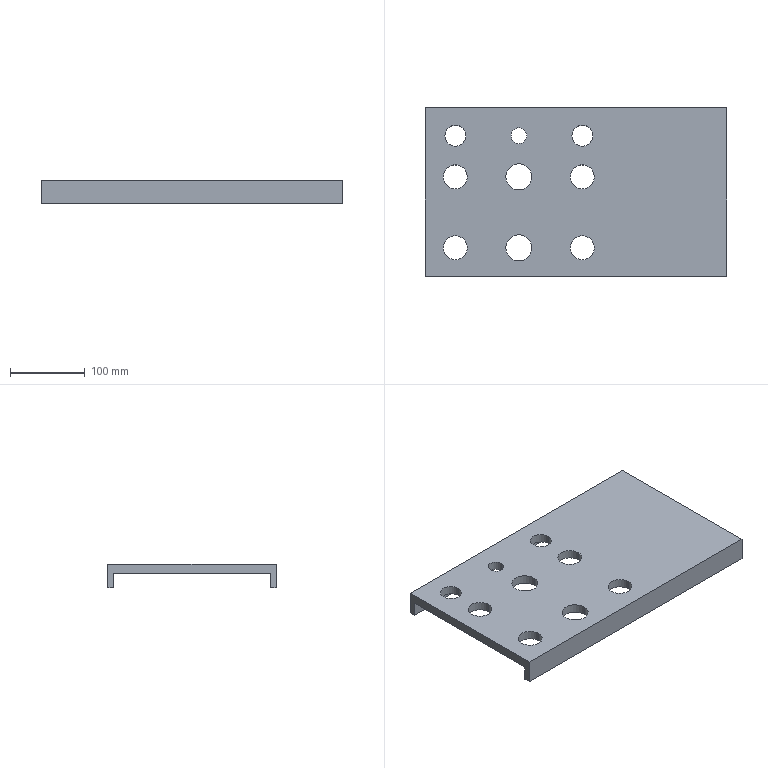Part | SolidWorks | features ICE 3, MoveFace 2, Extrusion 1 | 1 solid | 28 faces | box 403 x 225.5 x 32 mm | volume 1138849 mm3 | cylinder 18 | plane 10 | commonest cylinder face diameters 32 x8 28 x4 35 x4 21 x2
STEP:
#1=CARTESIAN_POINT('',(71.,80.,0.));
#2=VERTEX_POINT('',#1);
#3=CARTESIAN_POINT('',(99.,80.,0.));
#4=VERTEX_POINT('',#3);
#5=CARTESIAN_POINT('',(85.,80.,0.));
#6=DIRECTION('',(0.,0.,1.));
#7=DIRECTION('',(-1.,0.,0.));
#8=AXIS2_PLACEMENT_3D('',#5,#6,#7);
#9=CIRCLE('',#8,14.);
#10=EDGE_CURVE('',#2,#4,#9,.T.);
#11=ORIENTED_EDGE('',*,*,#10,.F.);
#12=CARTESIAN_POINT('',(71.,80.,12.));
#13=VERTEX_POINT('',#12);
#14=CARTESIAN_POINT('',(71.,80.,-0.001));
#15=DIRECTION('',(0.,0.,1.));
#16=VECTOR('',#15,1000.);
#17=LINE('',#14,#16);
#18=EDGE_CURVE('',#2,#13,#17,.T.);
#19=ORIENTED_EDGE('',*,*,#18,.T.);
#20=CARTESIAN_POINT('',(99.,80.,12.));
#21=VERTEX_POINT('',#20);
#22=CARTESIAN_POINT('',(85.,80.,12.));
#23=DIRECTION('',(0.,0.,1.));
#24=DIRECTION('',(1.,0.,0.));
#25=AXIS2_PLACEMENT_3D('',#22,#23,#24);
#26=CIRCLE('',#25,14.);
#27=EDGE_CURVE('',#13,#21,#26,.T.);
#28=ORIENTED_EDGE('',*,*,#27,.T.);
#29=CARTESIAN_POINT('',(99.,80.,-0.001));
#30=DIRECTION('',(0.,0.,1.));
#31=VECTOR('',#30,1000.);
#32=LINE('',#29,#31);
#33=EDGE_CURVE('',#4,#21,#32,.T.);
#34=ORIENTED_EDGE('',*,*,#33,.F.);
#35=EDGE_LOOP('',(#11,#19,#28,#34));
#36=FACE_OUTER_BOUND('',#35,.T.);
#37=CARTESIAN_POINT('',(85.,80.,-0.001));
#38=DIRECTION('',(0.,0.,1.));
#39=DIRECTION('',(1.,0.,0.));
#40=AXIS2_PLACEMENT_3D('',#37,#38,#39);
#41=CYLINDRICAL_SURFACE('',#40,14.);
#42=ADVANCED_FACE('',(#36),#41,.F.);
#43=CARTESIAN_POINT('',(-99.,80.,0.));
#44=VERTEX_POINT('',#43);
#45=CARTESIAN_POINT('',(-71.,80.,0.));
#46=VERTEX_POINT('',#45);
#47=CARTESIAN_POINT('',(-85.,80.,0.));
#48=DIRECTION('',(0.,0.,1.));
#49=DIRECTION('',(-1.,0.,0.));
#50=AXIS2_PLACEMENT_3D('',#47,#48,#49);
#51=CIRCLE('',#50,14.);
#52=EDGE_CURVE('',#44,#46,#51,.T.);
#53=ORIENTED_EDGE('',*,*,#52,.F.);
#54=CARTESIAN_POINT('',(-99.,80.,12.));
#55=VERTEX_POINT('',#54);
#56=CARTESIAN_POINT('',(-99.,80.,-0.001));
#57=DIRECTION('',(0.,0.,1.));
#58=VECTOR('',#57,1000.);
#59=LINE('',#56,#58);
#60=EDGE_CURVE('',#44,#55,#59,.T.);
#61=ORIENTED_EDGE('',*,*,#60,.T.);
#62=CARTESIAN_POINT('',(-71.,80.,12.));
#63=VERTEX_POINT('',#62);
#64=CARTESIAN_POINT('',(-85.,80.,12.));
#65=DIRECTION('',(0.,0.,1.));
#66=DIRECTION('',(1.,0.,0.));
#67=AXIS2_PLACEMENT_3D('',#64,#65,#66);
#68=CIRCLE('',#67,14.);
#69=EDGE_CURVE('',#55,#63,#68,.T.);
#70=ORIENTED_EDGE('',*,*,#69,.T.);
#71=CARTESIAN_POINT('',(-71.,80.,-0.001));
#72=DIRECTION('',(0.,0.,1.));
#73=VECTOR('',#72,1000.);
#74=LINE('',#71,#73);
#75=EDGE_CURVE('',#46,#63,#74,.T.);
#76=ORIENTED_EDGE('',*,*,#75,.F.);
#77=EDGE_LOOP('',(#53,#61,#70,#76));
#78=FACE_OUTER_BOUND('',#77,.T.);
#79=CARTESIAN_POINT('',(-85.,80.,-0.001));
#80=DIRECTION('',(0.,0.,1.));
#81=DIRECTION('',(1.,0.,0.));
#82=AXIS2_PLACEMENT_3D('',#79,#80,#81);
#83=CYLINDRICAL_SURFACE('',#82,14.);
#84=ADVANCED_FACE('',(#78),#83,.F.);
#85=CARTESIAN_POINT('',(-17.5,25.,0.));
#86=VERTEX_POINT('',#85);
#87=CARTESIAN_POINT('',(17.5,25.,0.));
#88=VERTEX_POINT('',#87);
#89=CARTESIAN_POINT('',(0.,25.,0.));
#90=DIRECTION('',(0.,0.,1.));
#91=DIRECTION('',(-1.,0.,0.));
#92=AXIS2_PLACEMENT_3D('',#89,#90,#91);
#93=CIRCLE('',#92,17.5);
#94=EDGE_CURVE('',#86,#88,#93,.T.);
#95=ORIENTED_EDGE('',*,*,#94,.F.);
#96=CARTESIAN_POINT('',(-17.5,25.,12.));
#97=VERTEX_POINT('',#96);
#98=CARTESIAN_POINT('',(-17.5,25.,-0.001));
#99=DIRECTION('',(0.,0.,1.));
#100=VECTOR('',#99,1000.);
#101=LINE('',#98,#100);
#102=EDGE_CURVE('',#86,#97,#101,.T.);
#103=ORIENTED_EDGE('',*,*,#102,.T.);
#104=CARTESIAN_POINT('',(17.5,25.,12.));
#105=VERTEX_POINT('',#104);
#106=CARTESIAN_POINT('',(0.,25.,12.));
#107=DIRECTION('',(0.,0.,1.));
#108=DIRECTION('',(1.,0.,0.));
#109=AXIS2_PLACEMENT_3D('',#106,#107,#108);
#110=CIRCLE('',#109,17.5);
#111=EDGE_CURVE('',#97,#105,#110,.T.);
#112=ORIENTED_EDGE('',*,*,#111,.T.);
#113=CARTESIAN_POINT('',(17.5,25.,-0.001));
#114=DIRECTION('',(0.,0.,1.));
#115=VECTOR('',#114,1000.);
#116=LINE('',#113,#115);
#117=EDGE_CURVE('',#88,#105,#116,.T.);
#118=ORIENTED_EDGE('',*,*,#117,.F.);
#119=EDGE_LOOP('',(#95,#103,#112,#118));
#120=FACE_OUTER_BOUND('',#119,.T.);
#121=CARTESIAN_POINT('',(0.,25.,-0.001));
#122=DIRECTION('',(0.,0.,1.));
#123=DIRECTION('',(1.,0.,0.));
#124=AXIS2_PLACEMENT_3D('',#121,#122,#123);
#125=CYLINDRICAL_SURFACE('',#124,17.5);
#126=ADVANCED_FACE('',(#120),#125,.F.);
#127=CARTESIAN_POINT('',(-101.,25.,0.));
#128=VERTEX_POINT('',#127);
#129=CARTESIAN_POINT('',(-69.,25.,0.));
#130=VERTEX_POINT('',#129);
#131=CARTESIAN_POINT('',(-85.,25.,0.));
#132=DIRECTION('',(0.,0.,1.));
#133=DIRECTION('',(-1.,0.,0.));
#134=AXIS2_PLACEMENT_3D('',#131,#132,#133);
#135=CIRCLE('',#134,16.);
#136=EDGE_CURVE('',#128,#130,#135,.T.);
#137=ORIENTED_EDGE('',*,*,#136,.F.);
#138=CARTESIAN_POINT('',(-101.,25.,12.));
#139=VERTEX_POINT('',#138);
#140=CARTESIAN_POINT('',(-101.,25.,-0.001));
#141=DIRECTION('',(0.,0.,1.));
#142=VECTOR('',#141,1000.);
#143=LINE('',#140,#142);
#144=EDGE_CURVE('',#128,#139,#143,.T.);
#145=ORIENTED_EDGE('',*,*,#144,.T.);
#146=CARTESIAN_POINT('',(-69.,25.,12.));
#147=VERTEX_POINT('',#146);
#148=CARTESIAN_POINT('',(-85.,25.,12.));
#149=DIRECTION('',(0.,0.,1.));
#150=DIRECTION('',(1.,0.,0.));
#151=AXIS2_PLACEMENT_3D('',#148,#149,#150);
#152=CIRCLE('',#151,16.);
#153=EDGE_CURVE('',#139,#147,#152,.T.);
#154=ORIENTED_EDGE('',*,*,#153,.T.);
#155=CARTESIAN_POINT('',(-69.,25.,-0.001));
#156=DIRECTION('',(0.,0.,1.));
#157=VECTOR('',#156,1000.);
#158=LINE('',#155,#157);
#159=EDGE_CURVE('',#130,#147,#158,.T.);
#160=ORIENTED_EDGE('',*,*,#159,.F.);
#161=EDGE_LOOP('',(#137,#145,#154,#160));
#162=FACE_OUTER_BOUND('',#161,.T.);
#163=CARTESIAN_POINT('',(-85.,25.,-0.001));
#164=DIRECTION('',(0.,0.,1.));
#165=DIRECTION('',(1.,0.,0.));
#166=AXIS2_PLACEMENT_3D('',#163,#164,#165);
#167=CYLINDRICAL_SURFACE('',#166,16.);
#168=ADVANCED_FACE('',(#162),#167,.F.);
#169=CARTESIAN_POINT('',(-101.,-70.,0.));
#170=VERTEX_POINT('',#169);
#171=CARTESIAN_POINT('',(-69.,-70.,0.));
#172=VERTEX_POINT('',#171);
#173=CARTESIAN_POINT('',(-85.,-70.,0.));
#174=DIRECTION('',(0.,0.,1.));
#175=DIRECTION('',(-1.,0.,0.));
#176=AXIS2_PLACEMENT_3D('',#173,#174,#175);
#177=CIRCLE('',#176,16.);
#178=EDGE_CURVE('',#170,#172,#177,.T.);
#179=ORIENTED_EDGE('',*,*,#178,.F.);
#180=CARTESIAN_POINT('',(-101.,-70.,12.));
#181=VERTEX_POINT('',#180);
#182=CARTESIAN_POINT('',(-101.,-70.,-0.001));
#183=DIRECTION('',(0.,0.,1.));
#184=VECTOR('',#183,1000.);
#185=LINE('',#182,#184);
#186=EDGE_CURVE('',#170,#181,#185,.T.);
#187=ORIENTED_EDGE('',*,*,#186,.T.);
#188=CARTESIAN_POINT('',(-69.,-70.,12.));
#189=VERTEX_POINT('',#188);
#190=CARTESIAN_POINT('',(-85.,-70.,12.));
#191=DIRECTION('',(0.,0.,1.));
#192=DIRECTION('',(1.,0.,0.));
#193=AXIS2_PLACEMENT_3D('',#190,#191,#192);
#194=CIRCLE('',#193,16.);
#195=EDGE_CURVE('',#181,#189,#194,.T.);
#196=ORIENTED_EDGE('',*,*,#195,.T.);
#197=CARTESIAN_POINT('',(-69.,-70.,-0.001));
#198=DIRECTION('',(0.,0.,1.));
#199=VECTOR('',#198,1000.);
#200=LINE('',#197,#199);
#201=EDGE_CURVE('',#172,#189,#200,.T.);
#202=ORIENTED_EDGE('',*,*,#201,.F.);
#203=EDGE_LOOP('',(#179,#187,#196,#202));
#204=FACE_OUTER_BOUND('',#203,.T.);
#205=CARTESIAN_POINT('',(-85.,-70.,-0.001));
#206=DIRECTION('',(0.,0.,1.));
#207=DIRECTION('',(1.,0.,0.));
#208=AXIS2_PLACEMENT_3D('',#205,#206,#207);
#209=CYLINDRICAL_SURFACE('',#208,16.);
#210=ADVANCED_FACE('',(#204),#209,.F.);
#211=CARTESIAN_POINT('',(69.,-70.,0.));
#212=VERTEX_POINT('',#211);
#213=CARTESIAN_POINT('',(101.,-70.,0.));
#214=VERTEX_POINT('',#213);
#215=CARTESIAN_POINT('',(85.,-70.,0.));
#216=DIRECTION('',(0.,0.,1.));
#217=DIRECTION('',(-1.,0.,0.));
#218=AXIS2_PLACEMENT_3D('',#215,#216,#217);
#219=CIRCLE('',#218,16.);
#220=EDGE_CURVE('',#212,#214,#219,.T.);
#221=ORIENTED_EDGE('',*,*,#220,.F.);
#222=CARTESIAN_POINT('',(69.,-70.,12.));
#223=VERTEX_POINT('',#222);
#224=CARTESIAN_POINT('',(69.,-70.,-0.001));
#225=DIRECTION('',(0.,0.,1.));
#226=VECTOR('',#225,1000.);
#227=LINE('',#224,#226);
#228=EDGE_CURVE('',#212,#223,#227,.T.);
#229=ORIENTED_EDGE('',*,*,#228,.T.);
#230=CARTESIAN_POINT('',(101.,-70.,12.));
#231=VERTEX_POINT('',#230);
#232=CARTESIAN_POINT('',(85.,-70.,12.));
#233=DIRECTION('',(0.,0.,1.));
#234=DIRECTION('',(1.,0.,0.));
#235=AXIS2_PLACEMENT_3D('',#232,#233,#234);
#236=CIRCLE('',#235,16.);
#237=EDGE_CURVE('',#223,#231,#236,.T.);
#238=ORIENTED_EDGE('',*,*,#237,.T.);
#239=CARTESIAN_POINT('',(101.,-70.,-0.001));
#240=DIRECTION('',(0.,0.,1.));
#241=VECTOR('',#240,1000.);
#242=LINE('',#239,#241);
#243=EDGE_CURVE('',#214,#231,#242,.T.);
#244=ORIENTED_EDGE('',*,*,#243,.F.);
#245=EDGE_LOOP('',(#221,#229,#238,#244));
#246=FACE_OUTER_BOUND('',#245,.T.);
#247=CARTESIAN_POINT('',(85.,-70.,-0.001));
#248=DIRECTION('',(0.,0.,1.));
#249=DIRECTION('',(1.,0.,0.));
#250=AXIS2_PLACEMENT_3D('',#247,#248,#249);
#251=CYLINDRICAL_SURFACE('',#250,16.);
#252=ADVANCED_FACE('',(#246),#251,.F.);
#253=CARTESIAN_POINT('',(-17.5,-70.,0.));
#254=VERTEX_POINT('',#253);
#255=CARTESIAN_POINT('',(17.5,-70.,0.));
#256=VERTEX_POINT('',#255);
#257=CARTESIAN_POINT('',(0.,-70.,0.));
#258=DIRECTION('',(0.,0.,1.));
#259=DIRECTION('',(-1.,0.,0.));
#260=AXIS2_PLACEMENT_3D('',#257,#258,#259);
#261=CIRCLE('',#260,17.5);
#262=EDGE_CURVE('',#254,#256,#261,.T.);
#263=ORIENTED_EDGE('',*,*,#262,.F.);
#264=CARTESIAN_POINT('',(-17.5,-70.,12.));
#265=VERTEX_POINT('',#264);
#266=CARTESIAN_POINT('',(-17.5,-70.,-0.001));
#267=DIRECTION('',(0.,0.,1.));
#268=VECTOR('',#267,1000.);
#269=LINE('',#266,#268);
#270=EDGE_CURVE('',#254,#265,#269,.T.);
#271=ORIENTED_EDGE('',*,*,#270,.T.);
#272=CARTESIAN_POINT('',(17.5,-70.,12.));
#273=VERTEX_POINT('',#272);
#274=CARTESIAN_POINT('',(0.,-70.,12.));
#275=DIRECTION('',(0.,0.,1.));
#276=DIRECTION('',(1.,0.,0.));
#277=AXIS2_PLACEMENT_3D('',#274,#275,#276);
#278=CIRCLE('',#277,17.5);
#279=EDGE_CURVE('',#265,#273,#278,.T.);
#280=ORIENTED_EDGE('',*,*,#279,.T.);
#281=CARTESIAN_POINT('',(17.5,-70.,-0.001));
#282=DIRECTION('',(0.,0.,1.));
#283=VECTOR('',#282,1000.);
#284=LINE('',#281,#283);
#285=EDGE_CURVE('',#256,#273,#284,.T.);
#286=ORIENTED_EDGE('',*,*,#285,.F.);
#287=EDGE_LOOP('',(#263,#271,#280,#286));
#288=FACE_OUTER_BOUND('',#287,.T.);
#289=CARTESIAN_POINT('',(0.,-70.,-0.001));
#290=DIRECTION('',(0.,0.,1.));
#291=DIRECTION('',(1.,0.,0.));
#292=AXIS2_PLACEMENT_3D('',#289,#290,#291);
#293=CYLINDRICAL_SURFACE('',#292,17.5);
#294=ADVANCED_FACE('',(#288),#293,.F.);
#295=CARTESIAN_POINT('',(69.,25.,0.));
#296=VERTEX_POINT('',#295);
#297=CARTESIAN_POINT('',(101.,25.,0.));
#298=VERTEX_POINT('',#297);
#299=CARTESIAN_POINT('',(85.,25.,0.));
#300=DIRECTION('',(0.,0.,1.));
#301=DIRECTION('',(-1.,0.,0.));
#302=AXIS2_PLACEMENT_3D('',#299,#300,#301);
#303=CIRCLE('',#302,16.);
#304=EDGE_CURVE('',#296,#298,#303,.T.);
#305=ORIENTED_EDGE('',*,*,#304,.F.);
#306=CARTESIAN_POINT('',(69.,25.,12.));
#307=VERTEX_POINT('',#306);
#308=CARTESIAN_POINT('',(69.,25.,-0.001));
#309=DIRECTION('',(0.,0.,1.));
#310=VECTOR('',#309,1000.);
#311=LINE('',#308,#310);
#312=EDGE_CURVE('',#296,#307,#311,.T.);
#313=ORIENTED_EDGE('',*,*,#312,.T.);
#314=CARTESIAN_POINT('',(101.,25.,12.));
#315=VERTEX_POINT('',#314);
#316=CARTESIAN_POINT('',(85.,25.,12.));
#317=DIRECTION('',(0.,0.,1.));
#318=DIRECTION('',(1.,0.,0.));
#319=AXIS2_PLACEMENT_3D('',#316,#317,#318);
#320=CIRCLE('',#319,16.);
#321=EDGE_CURVE('',#307,#315,#320,.T.);
#322=ORIENTED_EDGE('',*,*,#321,.T.);
#323=CARTESIAN_POINT('',(101.,25.,-0.001));
#324=DIRECTION('',(0.,0.,1.));
#325=VECTOR('',#324,1000.);
#326=LINE('',#323,#325);
#327=EDGE_CURVE('',#298,#315,#326,.T.);
#328=ORIENTED_EDGE('',*,*,#327,.F.);
#329=EDGE_LOOP('',(#305,#313,#322,#328));
#330=FACE_OUTER_BOUND('',#329,.T.);
#331=CARTESIAN_POINT('',(85.,25.,-0.001));
#332=DIRECTION('',(0.,0.,1.));
#333=DIRECTION('',(1.,0.,0.));
#334=AXIS2_PLACEMENT_3D('',#331,#332,#333);
#335=CYLINDRICAL_SURFACE('',#334,16.);
#336=ADVANCED_FACE('',(#330),#335,.F.);
#337=CARTESIAN_POINT('',(-10.5,80.,0.));
#338=VERTEX_POINT('',#337);
#339=CARTESIAN_POINT('',(10.5,80.,0.));
#340=VERTEX_POINT('',#339);
#341=CARTESIAN_POINT('',(0.,80.,0.));
#342=DIRECTION('',(0.,0.,1.));
#343=DIRECTION('',(-1.,0.,0.));
#344=AXIS2_PLACEMENT_3D('',#341,#342,#343);
#345=CIRCLE('',#344,10.5);
#346=EDGE_CURVE('',#338,#340,#345,.T.);
#347=ORIENTED_EDGE('',*,*,#346,.F.);
#348=CARTESIAN_POINT('',(-10.5,80.,12.));
#349=VERTEX_POINT('',#348);
#350=CARTESIAN_POINT('',(-10.5,80.,-0.001));
#351=DIRECTION('',(0.,0.,1.));
#352=VECTOR('',#351,1000.);
#353=LINE('',#350,#352);
#354=EDGE_CURVE('',#338,#349,#353,.T.);
#355=ORIENTED_EDGE('',*,*,#354,.T.);
#356=CARTESIAN_POINT('',(10.5,80.,12.));
#357=VERTEX_POINT('',#356);
#358=CARTESIAN_POINT('',(0.,80.,12.));
#359=DIRECTION('',(0.,0.,1.));
#360=DIRECTION('',(1.,0.,0.));
#361=AXIS2_PLACEMENT_3D('',#358,#359,#360);
#362=CIRCLE('',#361,10.5);
#363=EDGE_CURVE('',#349,#357,#362,.T.);
#364=ORIENTED_EDGE('',*,*,#363,.T.);
#365=CARTESIAN_POINT('',(10.5,80.,-0.001));
#366=DIRECTION('',(0.,0.,1.));
#367=VECTOR('',#366,1000.);
#368=LINE('',#365,#367);
#369=EDGE_CURVE('',#340,#357,#368,.T.);
#370=ORIENTED_EDGE('',*,*,#369,.F.);
#371=EDGE_LOOP('',(#347,#355,#364,#370));
#372=FACE_OUTER_BOUND('',#371,.T.);
#373=CARTESIAN_POINT('',(0.,80.,-0.001));
#374=DIRECTION('',(0.,0.,1.));
#375=DIRECTION('',(1.,0.,0.));
#376=AXIS2_PLACEMENT_3D('',#373,#374,#375);
#377=CYLINDRICAL_SURFACE('',#376,10.5);
#378=ADVANCED_FACE('',(#372),#377,.F.);
#379=CARTESIAN_POINT('',(85.,80.,0.));
#380=DIRECTION('',(0.,0.,1.));
#381=DIRECTION('',(-1.,0.,0.));
#382=AXIS2_PLACEMENT_3D('',#379,#380,#381);
#383=CIRCLE('',#382,14.);
#384=EDGE_CURVE('',#4,#2,#383,.T.);
#385=ORIENTED_EDGE('',*,*,#384,.T.);
#386=ORIENTED_EDGE('',*,*,#10,.T.);
#387=EDGE_LOOP('',(#385,#386));
#388=FACE_BOUND('',#387,.T.);
#389=CARTESIAN_POINT('',(-85.,80.,0.));
#390=DIRECTION('',(0.,0.,1.));
#391=DIRECTION('',(-1.,0.,0.));
#392=AXIS2_PLACEMENT_3D('',#389,#390,#391);
#393=CIRCLE('',#392,14.);
#394=EDGE_CURVE('',#46,#44,#393,.T.);
#395=ORIENTED_EDGE('',*,*,#394,.T.);
#396=ORIENTED_EDGE('',*,*,#52,.T.);
#397=EDGE_LOOP('',(#395,#396));
#398=FACE_BOUND('',#397,.T.);
#399=CARTESIAN_POINT('',(0.,25.,0.));
#400=DIRECTION('',(0.,0.,1.));
#401=DIRECTION('',(-1.,0.,0.));
#402=AXIS2_PLACEMENT_3D('',#399,#400,#401);
#403=CIRCLE('',#402,17.5);
#404=EDGE_CURVE('',#88,#86,#403,.T.);
#405=ORIENTED_EDGE('',*,*,#404,.T.);
#406=ORIENTED_EDGE('',*,*,#94,.T.);
#407=EDGE_LOOP('',(#405,#406));
#408=FACE_BOUND('',#407,.T.);
#409=CARTESIAN_POINT('',(-85.,25.,0.));
#410=DIRECTION('',(0.,0.,1.));
#411=DIRECTION('',(-1.,0.,0.));
#412=AXIS2_PLACEMENT_3D('',#409,#410,#411);
#413=CIRCLE('',#412,16.);
#414=EDGE_CURVE('',#130,#128,#413,.T.);
#415=ORIENTED_EDGE('',*,*,#414,.T.);
#416=ORIENTED_EDGE('',*,*,#136,.T.);
#417=EDGE_LOOP('',(#415,#416));
#418=FACE_BOUND('',#417,.T.);
#419=CARTESIAN_POINT('',(-85.,-70.,0.));
#420=DIRECTION('',(0.,0.,1.));
#421=DIRECTION('',(-1.,0.,0.));
#422=AXIS2_PLACEMENT_3D('',#419,#420,#421);
#423=CIRCLE('',#422,16.);
#424=EDGE_CURVE('',#172,#170,#423,.T.);
#425=ORIENTED_EDGE('',*,*,#424,.T.);
#426=ORIENTED_EDGE('',*,*,#178,.T.);
#427=EDGE_LOOP('',(#425,#426));
#428=FACE_BOUND('',#427,.T.);
#429=CARTESIAN_POINT('',(85.,-70.,0.));
#430=DIRECTION('',(0.,0.,1.));
#431=DIRECTION('',(-1.,0.,0.));
#432=AXIS2_PLACEMENT_3D('',#429,#430,#431);
#433=CIRCLE('',#432,16.);
#434=EDGE_CURVE('',#214,#212,#433,.T.);
#435=ORIENTED_EDGE('',*,*,#434,.T.);
#436=ORIENTED_EDGE('',*,*,#220,.T.);
#437=EDGE_LOOP('',(#435,#436));
#438=FACE_BOUND('',#437,.T.);
#439=CARTESIAN_POINT('',(0.,-70.,0.));
#440=DIRECTION('',(0.,0.,1.));
#441=DIRECTION('',(-1.,0.,0.));
#442=AXIS2_PLACEMENT_3D('',#439,#440,#441);
#443=CIRCLE('',#442,17.5);
#444=EDGE_CURVE('',#256,#254,#443,.T.);
#445=ORIENTED_EDGE('',*,*,#444,.T.);
#446=ORIENTED_EDGE('',*,*,#262,.T.);
#447=EDGE_LOOP('',(#445,#446));
#448=FACE_BOUND('',#447,.T.);
#449=CARTESIAN_POINT('',(85.,25.,0.));
#450=DIRECTION('',(0.,0.,1.));
#451=DIRECTION('',(-1.,0.,0.));
#452=AXIS2_PLACEMENT_3D('',#449,#450,#451);
#453=CIRCLE('',#452,16.);
#454=EDGE_CURVE('',#298,#296,#453,.T.);
#455=ORIENTED_EDGE('',*,*,#454,.T.);
#456=ORIENTED_EDGE('',*,*,#304,.T.);
#457=EDGE_LOOP('',(#455,#456));
#458=FACE_BOUND('',#457,.T.);
#459=CARTESIAN_POINT('',(0.,80.,0.));
#460=DIRECTION('',(0.,0.,1.));
#461=DIRECTION('',(-1.,0.,0.));
#462=AXIS2_PLACEMENT_3D('',#459,#460,#461);
#463=CIRCLE('',#462,10.5);
#464=EDGE_CURVE('',#340,#338,#463,.T.);
#465=ORIENTED_EDGE('',*,*,#464,.T.);
#466=ORIENTED_EDGE('',*,*,#346,.T.);
#467=EDGE_LOOP('',(#465,#466));
#468=FACE_BOUND('',#467,.T.);
#469=CARTESIAN_POINT('',(278.,-100.,0.));
#470=VERTEX_POINT('',#469);
#471=CARTESIAN_POINT('',(278.,109.5,0.));
#472=VERTEX_POINT('',#471);
#473=CARTESIAN_POINT('',(278.,-100.,0.));
#474=DIRECTION('',(0.,1.,0.));
#475=VECTOR('',#474,1000.);
#476=LINE('',#473,#475);
#477=EDGE_CURVE('',#470,#472,#476,.T.);
#478=ORIENTED_EDGE('',*,*,#477,.F.);
#479=CARTESIAN_POINT('',(-125.,-100.,0.));
#480=VERTEX_POINT('',#479);
#481=CARTESIAN_POINT('',(278.,-100.,0.));
#482=DIRECTION('',(1.,0.,0.));
#483=VECTOR('',#482,1000.);
#484=LINE('',#481,#483);
#485=EDGE_CURVE('',#480,#470,#484,.T.);
#486=ORIENTED_EDGE('',*,*,#485,.F.);
#487=CARTESIAN_POINT('',(-125.,109.5,0.));
#488=VERTEX_POINT('',#487);
#489=CARTESIAN_POINT('',(-125.,-100.,0.));
#490=DIRECTION('',(0.,-1.,0.));
#491=VECTOR('',#490,1000.);
#492=LINE('',#489,#491);
#493=EDGE_CURVE('',#488,#480,#492,.T.);
#494=ORIENTED_EDGE('',*,*,#493,.F.);
#495=CARTESIAN_POINT('',(-125.,109.5,0.));
#496=DIRECTION('',(-1.,0.,0.));
#497=VECTOR('',#496,1000.);
#498=LINE('',#495,#497);
#499=EDGE_CURVE('',#472,#488,#498,.T.);
#500=ORIENTED_EDGE('',*,*,#499,.F.);
#501=EDGE_LOOP('',(#478,#486,#494,#500));
#502=FACE_OUTER_BOUND('',#501,.T.);
#503=CARTESIAN_POINT('',(0.,0.,0.));
#504=DIRECTION('',(0.,0.,-1.));
#505=DIRECTION('',(-1.,0.,0.));
#506=AXIS2_PLACEMENT_3D('',#503,#504,#505);
#507=PLANE('',#506);
#508=ADVANCED_FACE('',(#388,#398,#408,#418,#428,#438,#448,#458,#468,#502),#507,.T.);
#509=CARTESIAN_POINT('',(278.,117.5,-20.));
#510=VERTEX_POINT('',#509);
#511=CARTESIAN_POINT('',(278.,117.5,12.));
#512=VERTEX_POINT('',#511);
#513=CARTESIAN_POINT('',(278.,117.5,12.));
#514=DIRECTION('',(0.,0.,1.));
#515=VECTOR('',#514,1000.);
#516=LINE('',#513,#515);
#517=EDGE_CURVE('',#510,#512,#516,.T.);
#518=ORIENTED_EDGE('',*,*,#517,.F.);
#519=CARTESIAN_POINT('',(-125.,117.5,-20.));
#520=VERTEX_POINT('',#519);
#521=CARTESIAN_POINT('',(-125.,117.5,-20.));
#522=DIRECTION('',(1.,0.,0.));
#523=VECTOR('',#522,1000.);
#524=LINE('',#521,#523);
#525=EDGE_CURVE('',#520,#510,#524,.T.);
#526=ORIENTED_EDGE('',*,*,#525,.F.);
#527=CARTESIAN_POINT('',(-125.,117.5,12.));
#528=VERTEX_POINT('',#527);
#529=CARTESIAN_POINT('',(-125.,117.5,12.));
#530=DIRECTION('',(0.,0.,-1.));
#531=VECTOR('',#530,1000.);
#532=LINE('',#529,#531);
#533=EDGE_CURVE('',#528,#520,#532,.T.);
#534=ORIENTED_EDGE('',*,*,#533,.F.);
#535=CARTESIAN_POINT('',(-125.,117.5,12.));
#536=DIRECTION('',(-1.,0.,0.));
#537=VECTOR('',#536,1000.);
#538=LINE('',#535,#537);
#539=EDGE_CURVE('',#512,#528,#538,.T.);
#540=ORIENTED_EDGE('',*,*,#539,.F.);
#541=EDGE_LOOP('',(#518,#526,#534,#540));
#542=FACE_OUTER_BOUND('',#541,.T.);
#543=CARTESIAN_POINT('',(-125.,117.5,12.));
#544=DIRECTION('',(0.,-1.,0.));
#545=DIRECTION('',(0.,0.,-1.));
#546=AXIS2_PLACEMENT_3D('',#543,#544,#545);
#547=PLANE('',#546);
#548=ADVANCED_FACE('',(#542),#547,.F.);
#549=ORIENTED_EDGE('',*,*,#533,.T.);
#550=CARTESIAN_POINT('',(-125.,109.5,-20.));
#551=VERTEX_POINT('',#550);
#552=CARTESIAN_POINT('',(-125.,117.5,-20.));
#553=DIRECTION('',(0.,1.,0.));
#554=VECTOR('',#553,1000.);
#555=LINE('',#552,#554);
#556=EDGE_CURVE('',#551,#520,#555,.T.);
#557=ORIENTED_EDGE('',*,*,#556,.F.);
#558=CARTESIAN_POINT('',(-125.,109.5,-20.));
#559=DIRECTION('',(0.,0.,1.));
#560=VECTOR('',#559,1000.);
#561=LINE('',#558,#560);
#562=EDGE_CURVE('',#551,#488,#561,.T.);
#563=ORIENTED_EDGE('',*,*,#562,.T.);
#564=ORIENTED_EDGE('',*,*,#493,.T.);
#565=CARTESIAN_POINT('',(-125.,-100.,-20.));
#566=VERTEX_POINT('',#565);
#567=CARTESIAN_POINT('',(-125.,-100.,-20.));
#568=DIRECTION('',(0.,0.,1.));
#569=VECTOR('',#568,1000.);
#570=LINE('',#567,#569);
#571=EDGE_CURVE('',#566,#480,#570,.T.);
#572=ORIENTED_EDGE('',*,*,#571,.F.);
#573=CARTESIAN_POINT('',(-125.,-108.,-20.));
#574=VERTEX_POINT('',#573);
#575=CARTESIAN_POINT('',(-125.,-108.,-20.));
#576=DIRECTION('',(0.,1.,0.));
#577=VECTOR('',#576,1000.);
#578=LINE('',#575,#577);
#579=EDGE_CURVE('',#574,#566,#578,.T.);
#580=ORIENTED_EDGE('',*,*,#579,.F.);
#581=CARTESIAN_POINT('',(-125.,-108.,12.));
#582=VERTEX_POINT('',#581);
#583=CARTESIAN_POINT('',(-125.,-108.,12.));
#584=DIRECTION('',(0.,0.,-1.));
#585=VECTOR('',#584,1000.);
#586=LINE('',#583,#585);
#587=EDGE_CURVE('',#582,#574,#586,.T.);
#588=ORIENTED_EDGE('',*,*,#587,.F.);
#589=CARTESIAN_POINT('',(-125.,-100.,12.));
#590=DIRECTION('',(0.,-1.,0.));
#591=VECTOR('',#590,1000.);
#592=LINE('',#589,#591);
#593=EDGE_CURVE('',#528,#582,#592,.T.);
#594=ORIENTED_EDGE('',*,*,#593,.F.);
#595=EDGE_LOOP('',(#549,#557,#563,#564,#572,#580,#588,#594));
#596=FACE_OUTER_BOUND('',#595,.T.);
#597=CARTESIAN_POINT('',(-125.,-100.,12.));
#598=DIRECTION('',(1.,0.,0.));
#599=DIRECTION('',(0.,0.,-1.));
#600=AXIS2_PLACEMENT_3D('',#597,#598,#599);
#601=PLANE('',#600);
#602=ADVANCED_FACE('',(#596),#601,.F.);
#603=ORIENTED_EDGE('',*,*,#587,.T.);
#604=CARTESIAN_POINT('',(278.,-108.,-20.));
#605=VERTEX_POINT('',#604);
#606=CARTESIAN_POINT('',(278.,-108.,-20.));
#607=DIRECTION('',(-1.,0.,0.));
#608=VECTOR('',#607,1000.);
#609=LINE('',#606,#608);
#610=EDGE_CURVE('',#605,#574,#609,.T.);
#611=ORIENTED_EDGE('',*,*,#610,.F.);
#612=CARTESIAN_POINT('',(278.,-108.,12.));
#613=VERTEX_POINT('',#612);
#614=CARTESIAN_POINT('',(278.,-108.,12.));
#615=DIRECTION('',(0.,0.,-1.));
#616=VECTOR('',#615,1000.);
#617=LINE('',#614,#616);
#618=EDGE_CURVE('',#613,#605,#617,.T.);
#619=ORIENTED_EDGE('',*,*,#618,.F.);
#620=CARTESIAN_POINT('',(-125.,-108.,12.));
#621=DIRECTION('',(1.,0.,0.));
#622=VECTOR('',#621,1000.);
#623=LINE('',#620,#622);
#624=EDGE_CURVE('',#582,#613,#623,.T.);
#625=ORIENTED_EDGE('',*,*,#624,.F.);
#626=EDGE_LOOP('',(#603,#611,#619,#625));
#627=FACE_OUTER_BOUND('',#626,.T.);
#628=CARTESIAN_POINT('',(-125.,-108.,12.));
#629=DIRECTION('',(0.,1.,0.));
#630=DIRECTION('',(0.,0.,1.));
#631=AXIS2_PLACEMENT_3D('',#628,#629,#630);
#632=PLANE('',#631);
#633=ADVANCED_FACE('',(#627),#632,.F.);
#634=CARTESIAN_POINT('',(85.,80.,12.));
#635=DIRECTION('',(0.,0.,1.));
#636=DIRECTION('',(1.,0.,0.));
#637=AXIS2_PLACEMENT_3D('',#634,#635,#636);
#638=CIRCLE('',#637,14.);
#639=EDGE_CURVE('',#21,#13,#638,.T.);
#640=ORIENTED_EDGE('',*,*,#639,.F.);
#641=ORIENTED_EDGE('',*,*,#27,.F.);
#642=EDGE_LOOP('',(#640,#641));
#643=FACE_BOUND('',#642,.T.);
#644=CARTESIAN_POINT('',(-85.,80.,12.));
#645=DIRECTION('',(0.,0.,1.));
#646=DIRECTION('',(1.,0.,0.));
#647=AXIS2_PLACEMENT_3D('',#644,#645,#646);
#648=CIRCLE('',#647,14.);
#649=EDGE_CURVE('',#63,#55,#648,.T.);
#650=ORIENTED_EDGE('',*,*,#649,.F.);
#651=ORIENTED_EDGE('',*,*,#69,.F.);
#652=EDGE_LOOP('',(#650,#651));
#653=FACE_BOUND('',#652,.T.);
#654=CARTESIAN_POINT('',(0.,25.,12.));
#655=DIRECTION('',(0.,0.,1.));
#656=DIRECTION('',(1.,0.,0.));
#657=AXIS2_PLACEMENT_3D('',#654,#655,#656);
#658=CIRCLE('',#657,17.5);
#659=EDGE_CURVE('',#105,#97,#658,.T.);
#660=ORIENTED_EDGE('',*,*,#659,.F.);
#661=ORIENTED_EDGE('',*,*,#111,.F.);
#662=EDGE_LOOP('',(#660,#661));
#663=FACE_BOUND('',#662,.T.);
#664=CARTESIAN_POINT('',(-85.,25.,12.));
#665=DIRECTION('',(0.,0.,1.));
#666=DIRECTION('',(1.,0.,0.));
#667=AXIS2_PLACEMENT_3D('',#664,#665,#666);
#668=CIRCLE('',#667,16.);
#669=EDGE_CURVE('',#147,#139,#668,.T.);
#670=ORIENTED_EDGE('',*,*,#669,.F.);
#671=ORIENTED_EDGE('',*,*,#153,.F.);
#672=EDGE_LOOP('',(#670,#671));
#673=FACE_BOUND('',#672,.T.);
#674=CARTESIAN_POINT('',(-85.,-70.,12.));
#675=DIRECTION('',(0.,0.,1.));
#676=DIRECTION('',(1.,0.,0.));
#677=AXIS2_PLACEMENT_3D('',#674,#675,#676);
#678=CIRCLE('',#677,16.);
#679=EDGE_CURVE('',#189,#181,#678,.T.);
#680=ORIENTED_EDGE('',*,*,#679,.F.);
#681=ORIENTED_EDGE('',*,*,#195,.F.);
#682=EDGE_LOOP('',(#680,#681));
#683=FACE_BOUND('',#682,.T.);
#684=CARTESIAN_POINT('',(85.,-70.,12.));
#685=DIRECTION('',(0.,0.,1.));
#686=DIRECTION('',(1.,0.,0.));
#687=AXIS2_PLACEMENT_3D('',#684,#685,#686);
#688=CIRCLE('',#687,16.);
#689=EDGE_CURVE('',#231,#223,#688,.T.);
#690=ORIENTED_EDGE('',*,*,#689,.F.);
#691=ORIENTED_EDGE('',*,*,#237,.F.);
#692=EDGE_LOOP('',(#690,#691));
#693=FACE_BOUND('',#692,.T.);
#694=CARTESIAN_POINT('',(0.,-70.,12.));
#695=DIRECTION('',(0.,0.,1.));
#696=DIRECTION('',(1.,0.,0.));
#697=AXIS2_PLACEMENT_3D('',#694,#695,#696);
#698=CIRCLE('',#697,17.5);
#699=EDGE_CURVE('',#273,#265,#698,.T.);
#700=ORIENTED_EDGE('',*,*,#699,.F.);
#701=ORIENTED_EDGE('',*,*,#279,.F.);
#702=EDGE_LOOP('',(#700,#701));
#703=FACE_BOUND('',#702,.T.);
#704=CARTESIAN_POINT('',(85.,25.,12.));
#705=DIRECTION('',(0.,0.,1.));
#706=DIRECTION('',(1.,0.,0.));
#707=AXIS2_PLACEMENT_3D('',#704,#705,#706);
#708=CIRCLE('',#707,16.);
#709=EDGE_CURVE('',#315,#307,#708,.T.);
#710=ORIENTED_EDGE('',*,*,#709,.F.);
#711=ORIENTED_EDGE('',*,*,#321,.F.);
#712=EDGE_LOOP('',(#710,#711));
#713=FACE_BOUND('',#712,.T.);
#714=CARTESIAN_POINT('',(0.,80.,12.));
#715=DIRECTION('',(0.,0.,1.));
#716=DIRECTION('',(1.,0.,0.));
#717=AXIS2_PLACEMENT_3D('',#714,#715,#716);
#718=CIRCLE('',#717,10.5);
#719=EDGE_CURVE('',#357,#349,#718,.T.);
#720=ORIENTED_EDGE('',*,*,#719,.F.);
#721=ORIENTED_EDGE('',*,*,#363,.F.);
#722=EDGE_LOOP('',(#720,#721));
#723=FACE_BOUND('',#722,.T.);
#724=ORIENTED_EDGE('',*,*,#624,.T.);
#725=CARTESIAN_POINT('',(278.,-100.,12.));
#726=DIRECTION('',(0.,-1.,0.));
#727=VECTOR('',#726,1000.);
#728=LINE('',#725,#727);
#729=EDGE_CURVE('',#512,#613,#728,.T.);
#730=ORIENTED_EDGE('',*,*,#729,.F.);
#731=ORIENTED_EDGE('',*,*,#539,.T.);
#732=ORIENTED_EDGE('',*,*,#593,.T.);
#733=EDGE_LOOP('',(#724,#730,#731,#732));
#734=FACE_OUTER_BOUND('',#733,.T.);
#735=CARTESIAN_POINT('',(0.,0.,12.));
#736=DIRECTION('',(0.,0.,-1.));
#737=DIRECTION('',(-1.,0.,0.));
#738=AXIS2_PLACEMENT_3D('',#735,#736,#737);
#739=PLANE('',#738);
#740=ADVANCED_FACE('',(#643,#653,#663,#673,#683,#693,#703,#713,#723,#734),#739,.F.);
#741=ORIENTED_EDGE('',*,*,#354,.F.);
#742=ORIENTED_EDGE('',*,*,#464,.F.);
#743=ORIENTED_EDGE('',*,*,#369,.T.);
#744=ORIENTED_EDGE('',*,*,#719,.T.);
#745=EDGE_LOOP('',(#741,#742,#743,#744));
#746=FACE_OUTER_BOUND('',#745,.T.);
#747=CARTESIAN_POINT('',(0.,80.,-0.001));
#748=DIRECTION('',(0.,0.,1.));
#749=DIRECTION('',(1.,0.,0.));
#750=AXIS2_PLACEMENT_3D('',#747,#748,#749);
#751=CYLINDRICAL_SURFACE('',#750,10.5);
#752=ADVANCED_FACE('',(#746),#751,.F.);
#753=ORIENTED_EDGE('',*,*,#312,.F.);
#754=ORIENTED_EDGE('',*,*,#454,.F.);
#755=ORIENTED_EDGE('',*,*,#327,.T.);
#756=ORIENTED_EDGE('',*,*,#709,.T.);
#757=EDGE_LOOP('',(#753,#754,#755,#756));
#758=FACE_OUTER_BOUND('',#757,.T.);
#759=CARTESIAN_POINT('',(85.,25.,-0.001));
#760=DIRECTION('',(0.,0.,1.));
#761=DIRECTION('',(1.,0.,0.));
#762=AXIS2_PLACEMENT_3D('',#759,#760,#761);
#763=CYLINDRICAL_SURFACE('',#762,16.);
#764=ADVANCED_FACE('',(#758),#763,.F.);
#765=ORIENTED_EDGE('',*,*,#270,.F.);
#766=ORIENTED_EDGE('',*,*,#444,.F.);
#767=ORIENTED_EDGE('',*,*,#285,.T.);
#768=ORIENTED_EDGE('',*,*,#699,.T.);
#769=EDGE_LOOP('',(#765,#766,#767,#768));
#770=FACE_OUTER_BOUND('',#769,.T.);
#771=CARTESIAN_POINT('',(0.,-70.,-0.001));
#772=DIRECTION('',(0.,0.,1.));
#773=DIRECTION('',(1.,0.,0.));
#774=AXIS2_PLACEMENT_3D('',#771,#772,#773);
#775=CYLINDRICAL_SURFACE('',#774,17.5);
#776=ADVANCED_FACE('',(#770),#775,.F.);
#777=ORIENTED_EDGE('',*,*,#228,.F.);
#778=ORIENTED_EDGE('',*,*,#434,.F.);
#779=ORIENTED_EDGE('',*,*,#243,.T.);
#780=ORIENTED_EDGE('',*,*,#689,.T.);
#781=EDGE_LOOP('',(#777,#778,#779,#780));
#782=FACE_OUTER_BOUND('',#781,.T.);
#783=CARTESIAN_POINT('',(85.,-70.,-0.001));
#784=DIRECTION('',(0.,0.,1.));
#785=DIRECTION('',(1.,0.,0.));
#786=AXIS2_PLACEMENT_3D('',#783,#784,#785);
#787=CYLINDRICAL_SURFACE('',#786,16.);
#788=ADVANCED_FACE('',(#782),#787,.F.);
#789=ORIENTED_EDGE('',*,*,#186,.F.);
#790=ORIENTED_EDGE('',*,*,#424,.F.);
#791=ORIENTED_EDGE('',*,*,#201,.T.);
#792=ORIENTED_EDGE('',*,*,#679,.T.);
#793=EDGE_LOOP('',(#789,#790,#791,#792));
#794=FACE_OUTER_BOUND('',#793,.T.);
#795=CARTESIAN_POINT('',(-85.,-70.,-0.001));
#796=DIRECTION('',(0.,0.,1.));
#797=DIRECTION('',(1.,0.,0.));
#798=AXIS2_PLACEMENT_3D('',#795,#796,#797);
#799=CYLINDRICAL_SURFACE('',#798,16.);
#800=ADVANCED_FACE('',(#794),#799,.F.);
#801=ORIENTED_EDGE('',*,*,#144,.F.);
#802=ORIENTED_EDGE('',*,*,#414,.F.);
#803=ORIENTED_EDGE('',*,*,#159,.T.);
#804=ORIENTED_EDGE('',*,*,#669,.T.);
#805=EDGE_LOOP('',(#801,#802,#803,#804));
#806=FACE_OUTER_BOUND('',#805,.T.);
#807=CARTESIAN_POINT('',(-85.,25.,-0.001));
#808=DIRECTION('',(0.,0.,1.));
#809=DIRECTION('',(1.,0.,0.));
#810=AXIS2_PLACEMENT_3D('',#807,#808,#809);
#811=CYLINDRICAL_SURFACE('',#810,16.);
#812=ADVANCED_FACE('',(#806),#811,.F.);
#813=ORIENTED_EDGE('',*,*,#102,.F.);
#814=ORIENTED_EDGE('',*,*,#404,.F.);
#815=ORIENTED_EDGE('',*,*,#117,.T.);
#816=ORIENTED_EDGE('',*,*,#659,.T.);
#817=EDGE_LOOP('',(#813,#814,#815,#816));
#818=FACE_OUTER_BOUND('',#817,.T.);
#819=CARTESIAN_POINT('',(0.,25.,-0.001));
#820=DIRECTION('',(0.,0.,1.));
#821=DIRECTION('',(1.,0.,0.));
#822=AXIS2_PLACEMENT_3D('',#819,#820,#821);
#823=CYLINDRICAL_SURFACE('',#822,17.5);
#824=ADVANCED_FACE('',(#818),#823,.F.);
#825=ORIENTED_EDGE('',*,*,#60,.F.);
#826=ORIENTED_EDGE('',*,*,#394,.F.);
#827=ORIENTED_EDGE('',*,*,#75,.T.);
#828=ORIENTED_EDGE('',*,*,#649,.T.);
#829=EDGE_LOOP('',(#825,#826,#827,#828));
#830=FACE_OUTER_BOUND('',#829,.T.);
#831=CARTESIAN_POINT('',(-85.,80.,-0.001));
#832=DIRECTION('',(0.,0.,1.));
#833=DIRECTION('',(1.,0.,0.));
#834=AXIS2_PLACEMENT_3D('',#831,#832,#833);
#835=CYLINDRICAL_SURFACE('',#834,14.);
#836=ADVANCED_FACE('',(#830),#835,.F.);
#837=ORIENTED_EDGE('',*,*,#18,.F.);
#838=ORIENTED_EDGE('',*,*,#384,.F.);
#839=ORIENTED_EDGE('',*,*,#33,.T.);
#840=ORIENTED_EDGE('',*,*,#639,.T.);
#841=EDGE_LOOP('',(#837,#838,#839,#840));
#842=FACE_OUTER_BOUND('',#841,.T.);
#843=CARTESIAN_POINT('',(85.,80.,-0.001));
#844=DIRECTION('',(0.,0.,1.));
#845=DIRECTION('',(1.,0.,0.));
#846=AXIS2_PLACEMENT_3D('',#843,#844,#845);
#847=CYLINDRICAL_SURFACE('',#846,14.);
#848=ADVANCED_FACE('',(#842),#847,.F.);
#849=ORIENTED_EDGE('',*,*,#729,.T.);
#850=ORIENTED_EDGE('',*,*,#618,.T.);
#851=CARTESIAN_POINT('',(278.,-100.,-20.));
#852=VERTEX_POINT('',#851);
#853=CARTESIAN_POINT('',(278.,-108.,-20.));
#854=DIRECTION('',(0.,-1.,0.));
#855=VECTOR('',#854,1000.);
#856=LINE('',#853,#855);
#857=EDGE_CURVE('',#852,#605,#856,.T.);
#858=ORIENTED_EDGE('',*,*,#857,.F.);
#859=CARTESIAN_POINT('',(278.,-100.,-20.));
#860=DIRECTION('',(0.,0.,1.));
#861=VECTOR('',#860,1000.);
#862=LINE('',#859,#861);
#863=EDGE_CURVE('',#852,#470,#862,.T.);
#864=ORIENTED_EDGE('',*,*,#863,.T.);
#865=ORIENTED_EDGE('',*,*,#477,.T.);
#866=CARTESIAN_POINT('',(278.,109.5,-20.));
#867=VERTEX_POINT('',#866);
#868=CARTESIAN_POINT('',(278.,109.5,-20.));
#869=DIRECTION('',(0.,0.,1.));
#870=VECTOR('',#869,1000.);
#871=LINE('',#868,#870);
#872=EDGE_CURVE('',#867,#472,#871,.T.);
#873=ORIENTED_EDGE('',*,*,#872,.F.);
#874=CARTESIAN_POINT('',(278.,117.5,-20.));
#875=DIRECTION('',(0.,-1.,0.));
#876=VECTOR('',#875,1000.);
#877=LINE('',#874,#876);
#878=EDGE_CURVE('',#510,#867,#877,.T.);
#879=ORIENTED_EDGE('',*,*,#878,.F.);
#880=ORIENTED_EDGE('',*,*,#517,.T.);
#881=EDGE_LOOP('',(#849,#850,#858,#864,#865,#873,#879,#880));
#882=FACE_OUTER_BOUND('',#881,.T.);
#883=CARTESIAN_POINT('',(278.,0.,0.));
#884=DIRECTION('',(-1.,0.,0.));
#885=DIRECTION('',(0.,0.,1.));
#886=AXIS2_PLACEMENT_3D('',#883,#884,#885);
#887=PLANE('',#886);
#888=ADVANCED_FACE('',(#882),#887,.F.);
#889=ORIENTED_EDGE('',*,*,#499,.T.);
#890=ORIENTED_EDGE('',*,*,#562,.F.);
#891=CARTESIAN_POINT('',(-125.,109.5,-20.));
#892=DIRECTION('',(-1.,0.,0.));
#893=VECTOR('',#892,1000.);
#894=LINE('',#891,#893);
#895=EDGE_CURVE('',#867,#551,#894,.T.);
#896=ORIENTED_EDGE('',*,*,#895,.F.);
#897=ORIENTED_EDGE('',*,*,#872,.T.);
#898=EDGE_LOOP('',(#889,#890,#896,#897));
#899=FACE_OUTER_BOUND('',#898,.T.);
#900=CARTESIAN_POINT('',(-125.,109.5,-20.));
#901=DIRECTION('',(0.,1.,0.));
#902=DIRECTION('',(-1.,0.,0.));
#903=AXIS2_PLACEMENT_3D('',#900,#901,#902);
#904=PLANE('',#903);
#905=ADVANCED_FACE('',(#899),#904,.F.);
#906=ORIENTED_EDGE('',*,*,#556,.T.);
#907=ORIENTED_EDGE('',*,*,#525,.T.);
#908=ORIENTED_EDGE('',*,*,#878,.T.);
#909=ORIENTED_EDGE('',*,*,#895,.T.);
#910=EDGE_LOOP('',(#906,#907,#908,#909));
#911=FACE_OUTER_BOUND('',#910,.T.);
#912=CARTESIAN_POINT('',(0.,0.,-20.));
#913=DIRECTION('',(0.,0.,1.));
#914=DIRECTION('',(1.,0.,0.));
#915=AXIS2_PLACEMENT_3D('',#912,#913,#914);
#916=PLANE('',#915);
#917=ADVANCED_FACE('',(#911),#916,.F.);
#918=ORIENTED_EDGE('',*,*,#485,.T.);
#919=ORIENTED_EDGE('',*,*,#863,.F.);
#920=CARTESIAN_POINT('',(278.,-100.,-20.));
#921=DIRECTION('',(1.,0.,0.));
#922=VECTOR('',#921,1000.);
#923=LINE('',#920,#922);
#924=EDGE_CURVE('',#566,#852,#923,.T.);
#925=ORIENTED_EDGE('',*,*,#924,.F.);
#926=ORIENTED_EDGE('',*,*,#571,.T.);
#927=EDGE_LOOP('',(#918,#919,#925,#926));
#928=FACE_OUTER_BOUND('',#927,.T.);
#929=CARTESIAN_POINT('',(278.,-100.,-20.));
#930=DIRECTION('',(0.,-1.,0.));
#931=DIRECTION('',(0.,0.,-1.));
#932=AXIS2_PLACEMENT_3D('',#929,#930,#931);
#933=PLANE('',#932);
#934=ADVANCED_FACE('',(#928),#933,.F.);
#935=ORIENTED_EDGE('',*,*,#857,.T.);
#936=ORIENTED_EDGE('',*,*,#610,.T.);
#937=ORIENTED_EDGE('',*,*,#579,.T.);
#938=ORIENTED_EDGE('',*,*,#924,.T.);
#939=EDGE_LOOP('',(#935,#936,#937,#938));
#940=FACE_OUTER_BOUND('',#939,.T.);
#941=CARTESIAN_POINT('',(0.,0.,-20.));
#942=DIRECTION('',(0.,0.,1.));
#943=DIRECTION('',(1.,0.,0.));
#944=AXIS2_PLACEMENT_3D('',#941,#942,#943);
#945=PLANE('',#944);
#946=ADVANCED_FACE('',(#940),#945,.F.);
#947=CLOSED_SHELL('',(#42,#84,#126,#168,#210,#252,#294,#336,#378,#508,#548,#602,#633,#740,#752,#764,#776,#788,#800,#812,#824,#836,#848,#888,#905,#917,#934,#946));
#948=MANIFOLD_SOLID_BREP('',#947);
#949=CARTESIAN_POINT('',(0.,0.,0.));
#950=DIRECTION('',(0.,0.,1.));
#951=DIRECTION('',(1.,0.,0.));
#952=AXIS2_PLACEMENT_3D('',#949,#950,#951);
#953=(LENGTH_UNIT()NAMED_UNIT(*)SI_UNIT(.MILLI.,.METRE.));
#954=UNCERTAINTY_MEASURE_WITH_UNIT(LENGTH_MEASURE(0.00001),#953,'','');
#955=(NAMED_UNIT(*)PLANE_ANGLE_UNIT()SI_UNIT($,.RADIAN.));
#956=(NAMED_UNIT(*)SI_UNIT($,.STERADIAN.)SOLID_ANGLE_UNIT());
#957=(GEOMETRIC_REPRESENTATION_CONTEXT(3)GLOBAL_UNCERTAINTY_ASSIGNED_CONTEXT((#954))GLOBAL_UNIT_ASSIGNED_CONTEXT((#953,#955,#956))REPRESENTATION_CONTEXT('',''));
#958=ADVANCED_BREP_SHAPE_REPRESENTATION('',(#948,#952),#957);